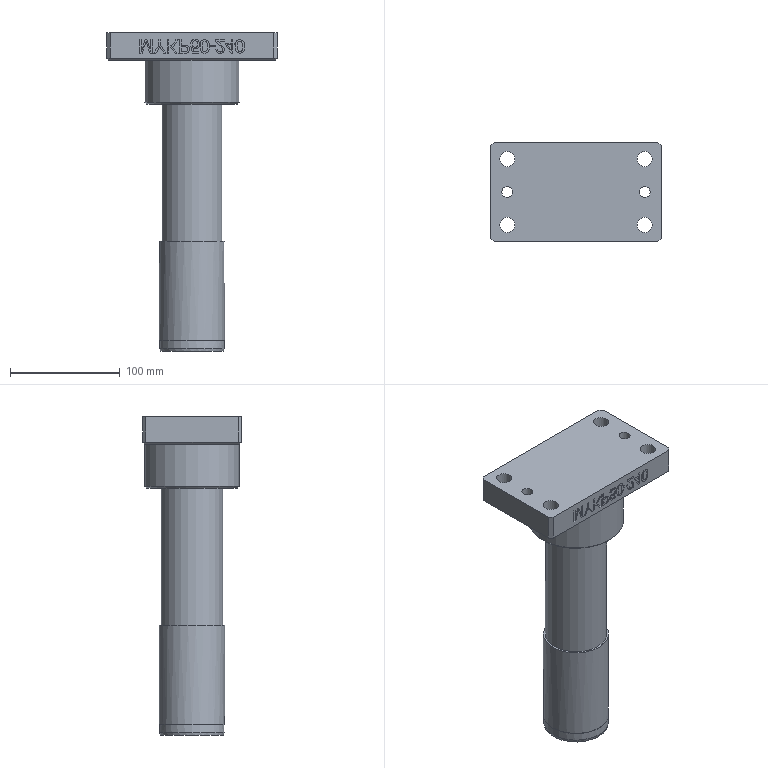Part | NX | features MI_MYKP_0875 2 | 1 solid | 184 faces | box 155 x 90 x 290 mm | volume 1136457 mm3 | plane 138 | cylinder 42 | cone 4 | commonest cylinder face diameters 14 x4 5.206 x2 6.212 x2 6.23 x2 6.303 x2 8.287 x2